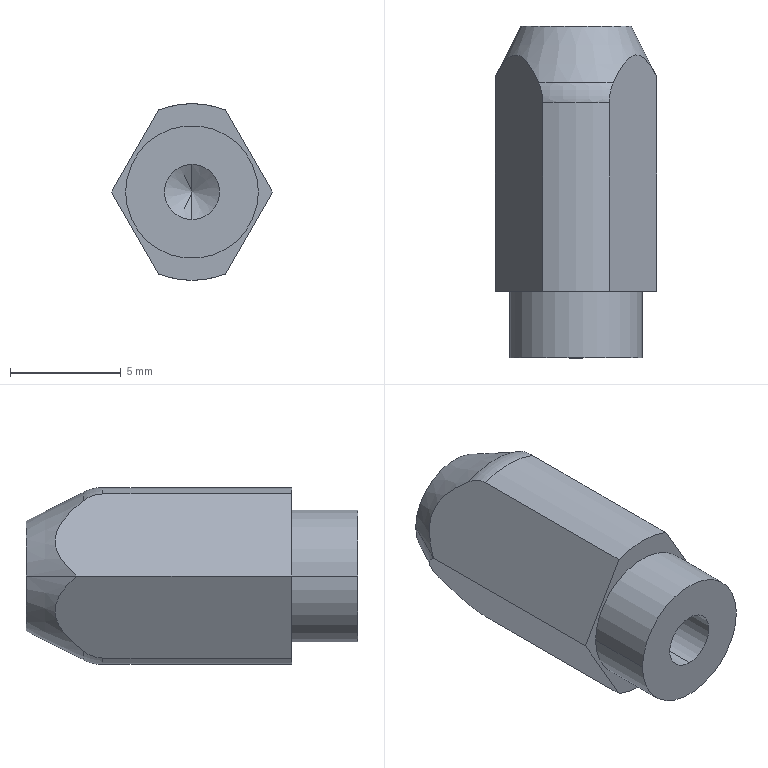Part | SolidWorks | features Fillet 1, HoleWzd 1, ICE 1, Revolution 1 | 1 solid | 19 faces | box 7.282 x 15 x 8 mm | volume 482.004 mm3 | plane 7 | cylinder 6 | cone 4 | torus 2 | commonest cylinder face diameters 2.5 x2 6 x2 8 x2
STEP:
#1=CARTESIAN_POINT('',(0.,10.,1.25));
#2=VERTEX_POINT('',#1);
#3=CARTESIAN_POINT('',(0.,10.,-1.25));
#4=VERTEX_POINT('',#3);
#5=CARTESIAN_POINT('',(0.,10.,0.));
#6=DIRECTION('',(0.,-1.,0.));
#7=DIRECTION('',(0.,0.,-1.));
#8=AXIS2_PLACEMENT_3D('',#5,#6,#7);
#9=CIRCLE('',#8,1.25);
#10=EDGE_CURVE('',#2,#4,#9,.T.);
#11=ORIENTED_EDGE('',*,*,#10,.F.);
#12=CARTESIAN_POINT('',(0.,0.,1.25));
#13=VERTEX_POINT('',#12);
#14=CARTESIAN_POINT('',(0.,0.,1.25));
#15=DIRECTION('',(0.,-1.,0.));
#16=VECTOR('',#15,1000.);
#17=LINE('',#14,#16);
#18=EDGE_CURVE('',#2,#13,#17,.T.);
#19=ORIENTED_EDGE('',*,*,#18,.T.);
#20=CARTESIAN_POINT('',(0.,0.,-1.25));
#21=VERTEX_POINT('',#20);
#22=CARTESIAN_POINT('',(0.,0.,0.));
#23=DIRECTION('',(0.,-1.,0.));
#24=DIRECTION('',(0.,0.,-1.));
#25=AXIS2_PLACEMENT_3D('',#22,#23,#24);
#26=CIRCLE('',#25,1.25);
#27=EDGE_CURVE('',#13,#21,#26,.T.);
#28=ORIENTED_EDGE('',*,*,#27,.T.);
#29=CARTESIAN_POINT('',(0.,0.,-1.25));
#30=DIRECTION('',(0.,-1.,0.));
#31=VECTOR('',#30,1000.);
#32=LINE('',#29,#31);
#33=EDGE_CURVE('',#4,#21,#32,.T.);
#34=ORIENTED_EDGE('',*,*,#33,.F.);
#35=EDGE_LOOP('',(#11,#19,#28,#34));
#36=FACE_OUTER_BOUND('',#35,.T.);
#37=CARTESIAN_POINT('',(0.,0.,0.));
#38=DIRECTION('',(0.,-1.,0.));
#39=DIRECTION('',(0.,0.,-1.));
#40=AXIS2_PLACEMENT_3D('',#37,#38,#39);
#41=CYLINDRICAL_SURFACE('',#40,1.25);
#42=ADVANCED_FACE('',(#36),#41,.F.);
#43=CARTESIAN_POINT('',(0.,10.751,0.));
#44=VERTEX_POINT('',#43);
#45=CARTESIAN_POINT('',(0.,10.,-1.25));
#46=DIRECTION('',(0.,-0.515,-0.8572));
#47=VECTOR('',#46,1000.);
#48=LINE('',#45,#47);
#49=EDGE_CURVE('',#44,#4,#48,.T.);
#50=ORIENTED_EDGE('',*,*,#49,.F.);
#51=CARTESIAN_POINT('',(0.,10.,1.25));
#52=DIRECTION('',(0.,-0.515,0.8572));
#53=VECTOR('',#52,1000.);
#54=LINE('',#51,#53);
#55=EDGE_CURVE('',#44,#2,#54,.T.);
#56=ORIENTED_EDGE('',*,*,#55,.T.);
#57=ORIENTED_EDGE('',*,*,#10,.T.);
#58=EDGE_LOOP('',(#50,#56,#57));
#59=FACE_OUTER_BOUND('',#58,.T.);
#60=CARTESIAN_POINT('',(0.,10.,0.));
#61=DIRECTION('',(0.,-1.,0.));
#62=DIRECTION('',(0.,0.,-1.));
#63=AXIS2_PLACEMENT_3D('',#60,#61,#62);
#64=CONICAL_SURFACE('',#63,1.25,1.03);
#65=ADVANCED_FACE('',(#59),#64,.F.);
#66=CARTESIAN_POINT('',(3.,3.,0.));
#67=VERTEX_POINT('',#66);
#68=CARTESIAN_POINT('',(-3.,3.,0.));
#69=VERTEX_POINT('',#68);
#70=CARTESIAN_POINT('',(0.,3.,0.));
#71=DIRECTION('',(0.,-1.,0.));
#72=DIRECTION('',(1.,0.,0.));
#73=AXIS2_PLACEMENT_3D('',#70,#71,#72);
#74=CIRCLE('',#73,3.);
#75=EDGE_CURVE('',#67,#69,#74,.T.);
#76=ORIENTED_EDGE('',*,*,#75,.T.);
#77=CARTESIAN_POINT('',(-3.,0.,0.));
#78=VERTEX_POINT('',#77);
#79=CARTESIAN_POINT('',(-3.,0.,0.));
#80=DIRECTION('',(0.,-1.,0.));
#81=VECTOR('',#80,1000.);
#82=LINE('',#79,#81);
#83=EDGE_CURVE('',#69,#78,#82,.T.);
#84=ORIENTED_EDGE('',*,*,#83,.T.);
#85=CARTESIAN_POINT('',(3.,0.,0.));
#86=VERTEX_POINT('',#85);
#87=CARTESIAN_POINT('',(0.,0.,0.));
#88=DIRECTION('',(0.,-1.,0.));
#89=DIRECTION('',(1.,0.,0.));
#90=AXIS2_PLACEMENT_3D('',#87,#88,#89);
#91=CIRCLE('',#90,3.);
#92=EDGE_CURVE('',#86,#78,#91,.T.);
#93=ORIENTED_EDGE('',*,*,#92,.F.);
#94=CARTESIAN_POINT('',(3.,0.,0.));
#95=DIRECTION('',(0.,-1.,0.));
#96=VECTOR('',#95,1000.);
#97=LINE('',#94,#96);
#98=EDGE_CURVE('',#67,#86,#97,.T.);
#99=ORIENTED_EDGE('',*,*,#98,.F.);
#100=EDGE_LOOP('',(#76,#84,#93,#99));
#101=FACE_OUTER_BOUND('',#100,.T.);
#102=CARTESIAN_POINT('',(0.,0.,0.));
#103=DIRECTION('',(0.,-1.,0.));
#104=DIRECTION('',(1.,0.,0.));
#105=AXIS2_PLACEMENT_3D('',#102,#103,#104);
#106=CYLINDRICAL_SURFACE('',#105,3.);
#107=ADVANCED_FACE('',(#101),#106,.T.);
#108=CARTESIAN_POINT('',(2.5,15.,0.));
#109=VERTEX_POINT('',#108);
#110=CARTESIAN_POINT('',(-2.5,15.,0.));
#111=VERTEX_POINT('',#110);
#112=CARTESIAN_POINT('',(0.,15.,0.));
#113=DIRECTION('',(0.,-1.,0.));
#114=DIRECTION('',(1.,0.,0.));
#115=AXIS2_PLACEMENT_3D('',#112,#113,#114);
#116=CIRCLE('',#115,2.5);
#117=EDGE_CURVE('',#109,#111,#116,.T.);
#118=ORIENTED_EDGE('',*,*,#117,.T.);
#119=CARTESIAN_POINT('',(-3.641,12.718,0.));
#120=VERTEX_POINT('',#119);
#121=CARTESIAN_POINT('',(-4.,12.,0.));
#122=DIRECTION('',(-0.4472,-0.8944,0.));
#123=VECTOR('',#122,1000.);
#124=LINE('',#121,#123);
#125=EDGE_CURVE('',#111,#120,#124,.T.);
#126=ORIENTED_EDGE('',*,*,#125,.T.);
#127=CARTESIAN_POINT('',(-1.68,12.422,3.396));
#128=VERTEX_POINT('',#127);
#129=CARTESIAN_POINT('',(-1.68,12.422,3.396));
#130=CARTESIAN_POINT('',(-1.745,12.566,3.284));
#131=CARTESIAN_POINT('',(-1.812,12.705,3.168));
#132=CARTESIAN_POINT('',(-1.953,12.972,2.924));
#133=CARTESIAN_POINT('',(-2.026,13.099,2.796));
#134=CARTESIAN_POINT('',(-2.182,13.329,2.527));
#135=CARTESIAN_POINT('',(-2.264,13.432,2.385));
#136=CARTESIAN_POINT('',(-2.44,13.597,2.079));
#137=CARTESIAN_POINT('',(-2.533,13.656,1.92));
#138=CARTESIAN_POINT('',(-2.727,13.706,1.584));
#139=CARTESIAN_POINT('',(-2.823,13.694,1.417));
#140=CARTESIAN_POINT('',(-3.013,13.605,1.088));
#141=CARTESIAN_POINT('',(-3.102,13.53,0.9338));
#142=CARTESIAN_POINT('',(-3.271,13.342,0.6408));
#143=CARTESIAN_POINT('',(-3.351,13.229,0.5025));
#144=CARTESIAN_POINT('',(-3.501,12.986,0.2421));
#145=CARTESIAN_POINT('',(-3.572,12.855,0.1188));
#146=CARTESIAN_POINT('',(-3.641,12.718,0.));
#147=B_SPLINE_CURVE_WITH_KNOTS('',3,(#129,#130,#131,#132,#133,#134,#135,#136,#137,#138,#139,#140,#141,#142,#143,#144,#145,#146),.UNSPECIFIED.,.F.,.F.,(4,2,2,2,2,2,2,2,4),(0.0005548,0.001135,0.001715,0.002295,0.002875,0.003455,0.004035,0.004615,0.005195),.UNSPECIFIED.);
#148=EDGE_CURVE('',#128,#120,#147,.T.);
#149=ORIENTED_EDGE('',*,*,#148,.F.);
#150=CARTESIAN_POINT('',(1.68,12.422,3.396));
#151=VERTEX_POINT('',#150);
#152=CARTESIAN_POINT('',(0.,12.422,0.));
#153=DIRECTION('',(0.,1.,0.));
#154=DIRECTION('',(-1.,0.,0.));
#155=AXIS2_PLACEMENT_3D('',#152,#153,#154);
#156=CIRCLE('',#155,3.789);
#157=EDGE_CURVE('',#128,#151,#156,.T.);
#158=ORIENTED_EDGE('',*,*,#157,.T.);
#159=CARTESIAN_POINT('',(3.641,12.718,0.));
#160=VERTEX_POINT('',#159);
#161=CARTESIAN_POINT('',(3.641,12.718,0.));
#162=CARTESIAN_POINT('',(3.572,12.856,0.1189));
#163=CARTESIAN_POINT('',(3.501,12.986,0.242));
#164=CARTESIAN_POINT('',(3.351,13.228,0.5015));
#165=CARTESIAN_POINT('',(3.273,13.339,0.6376));
#166=CARTESIAN_POINT('',(3.103,13.529,0.9318));
#167=CARTESIAN_POINT('',(3.012,13.605,1.089));
#168=CARTESIAN_POINT('',(2.87,13.672,1.335));
#169=CARTESIAN_POINT('',(2.821,13.686,1.42));
#170=CARTESIAN_POINT('',(2.724,13.697,1.587));
#171=CARTESIAN_POINT('',(2.676,13.693,1.671));
#172=CARTESIAN_POINT('',(2.58,13.668,1.837));
#173=CARTESIAN_POINT('',(2.532,13.647,1.921));
#174=CARTESIAN_POINT('',(2.439,13.589,2.082));
#175=CARTESIAN_POINT('',(2.394,13.554,2.16));
#176=CARTESIAN_POINT('',(2.262,13.43,2.388));
#177=CARTESIAN_POINT('',(2.179,13.325,2.532));
#178=CARTESIAN_POINT('',(1.947,12.981,2.935));
#179=CARTESIAN_POINT('',(1.81,12.71,3.172));
#180=CARTESIAN_POINT('',(1.68,12.422,3.396));
#181=B_SPLINE_CURVE_WITH_KNOTS('',3,(#161,#162,#163,#164,#165,#166,#167,#168,#169,#170,#171,#172,#173,#174,#175,#176,#177,#178,#179,#180),.UNSPECIFIED.,.F.,.F.,(4,2,2,2,2,2,2,2,2,4),(0.000000324,0.0005776,0.001155,0.001732,0.002021,0.002309,0.002598,0.002887,0.003464,0.004619),.UNSPECIFIED.);
#182=EDGE_CURVE('',#160,#151,#181,.T.);
#183=ORIENTED_EDGE('',*,*,#182,.F.);
#184=CARTESIAN_POINT('',(4.,12.,0.));
#185=DIRECTION('',(0.4472,-0.8944,0.));
#186=VECTOR('',#185,1000.);
#187=LINE('',#184,#186);
#188=EDGE_CURVE('',#109,#160,#187,.T.);
#189=ORIENTED_EDGE('',*,*,#188,.F.);
#190=EDGE_LOOP('',(#118,#126,#149,#158,#183,#189));
#191=FACE_OUTER_BOUND('',#190,.T.);
#192=CARTESIAN_POINT('',(0.,12.,0.));
#193=DIRECTION('',(0.,-1.,0.));
#194=DIRECTION('',(1.,0.,0.));
#195=AXIS2_PLACEMENT_3D('',#192,#193,#194);
#196=CONICAL_SURFACE('',#195,4.,0.4636);
#197=ADVANCED_FACE('',(#191),#196,.T.);
#198=CARTESIAN_POINT('',(1.5,3.,3.708));
#199=VERTEX_POINT('',#198);
#200=CARTESIAN_POINT('',(1.5,11.528,3.708));
#201=VERTEX_POINT('',#200);
#202=CARTESIAN_POINT('',(1.5,0.,3.708));
#203=DIRECTION('',(0.,1.,0.));
#204=VECTOR('',#203,1000.);
#205=LINE('',#202,#204);
#206=EDGE_CURVE('',#199,#201,#205,.T.);
#207=ORIENTED_EDGE('',*,*,#206,.T.);
#208=CARTESIAN_POINT('',(-1.5,11.528,3.708));
#209=VERTEX_POINT('',#208);
#210=CARTESIAN_POINT('',(0.,11.528,0.));
#211=DIRECTION('',(0.,-1.,0.));
#212=DIRECTION('',(-1.,0.,0.));
#213=AXIS2_PLACEMENT_3D('',#210,#211,#212);
#214=CIRCLE('',#213,4.);
#215=EDGE_CURVE('',#201,#209,#214,.T.);
#216=ORIENTED_EDGE('',*,*,#215,.T.);
#217=CARTESIAN_POINT('',(-1.5,3.,3.708));
#218=VERTEX_POINT('',#217);
#219=CARTESIAN_POINT('',(-1.5,0.,3.708));
#220=DIRECTION('',(0.,1.,0.));
#221=VECTOR('',#220,1000.);
#222=LINE('',#219,#221);
#223=EDGE_CURVE('',#218,#209,#222,.T.);
#224=ORIENTED_EDGE('',*,*,#223,.F.);
#225=CARTESIAN_POINT('',(0.,3.,0.));
#226=DIRECTION('',(0.,-1.,0.));
#227=DIRECTION('',(1.,0.,0.));
#228=AXIS2_PLACEMENT_3D('',#225,#226,#227);
#229=CIRCLE('',#228,4.);
#230=EDGE_CURVE('',#199,#218,#229,.T.);
#231=ORIENTED_EDGE('',*,*,#230,.F.);
#232=EDGE_LOOP('',(#207,#216,#224,#231));
#233=FACE_OUTER_BOUND('',#232,.T.);
#234=CARTESIAN_POINT('',(0.,0.,0.));
#235=DIRECTION('',(0.,-1.,0.));
#236=DIRECTION('',(1.,0.,0.));
#237=AXIS2_PLACEMENT_3D('',#234,#235,#236);
#238=CYLINDRICAL_SURFACE('',#237,4.);
#239=ADVANCED_FACE('',(#233),#238,.T.);
#240=CARTESIAN_POINT('',(0.,0.,0.));
#241=DIRECTION('',(0.,-1.,0.));
#242=DIRECTION('',(0.,0.,-1.));
#243=AXIS2_PLACEMENT_3D('',#240,#241,#242);
#244=CIRCLE('',#243,1.25);
#245=EDGE_CURVE('',#21,#13,#244,.T.);
#246=ORIENTED_EDGE('',*,*,#245,.F.);
#247=ORIENTED_EDGE('',*,*,#27,.F.);
#248=EDGE_LOOP('',(#246,#247));
#249=FACE_BOUND('',#248,.T.);
#250=ORIENTED_EDGE('',*,*,#92,.T.);
#251=CARTESIAN_POINT('',(0.,0.,0.));
#252=DIRECTION('',(0.,-1.,0.));
#253=DIRECTION('',(1.,0.,0.));
#254=AXIS2_PLACEMENT_3D('',#251,#252,#253);
#255=CIRCLE('',#254,3.);
#256=EDGE_CURVE('',#78,#86,#255,.T.);
#257=ORIENTED_EDGE('',*,*,#256,.T.);
#258=EDGE_LOOP('',(#250,#257));
#259=FACE_OUTER_BOUND('',#258,.T.);
#260=CARTESIAN_POINT('',(3.,0.,0.));
#261=DIRECTION('',(0.,-1.,0.));
#262=DIRECTION('',(1.,0.,0.));
#263=AXIS2_PLACEMENT_3D('',#260,#261,#262);
#264=PLANE('',#263);
#265=ADVANCED_FACE('',(#249,#259),#264,.T.);
#266=ORIENTED_EDGE('',*,*,#117,.F.);
#267=CARTESIAN_POINT('',(0.,15.,0.));
#268=DIRECTION('',(0.,-1.,0.));
#269=DIRECTION('',(1.,0.,0.));
#270=AXIS2_PLACEMENT_3D('',#267,#268,#269);
#271=CIRCLE('',#270,2.5);
#272=EDGE_CURVE('',#111,#109,#271,.T.);
#273=ORIENTED_EDGE('',*,*,#272,.F.);
#274=EDGE_LOOP('',(#266,#273));
#275=FACE_OUTER_BOUND('',#274,.T.);
#276=CARTESIAN_POINT('',(0.,15.,0.));
#277=DIRECTION('',(0.,1.,0.));
#278=DIRECTION('',(-1.,0.,0.));
#279=AXIS2_PLACEMENT_3D('',#276,#277,#278);
#280=PLANE('',#279);
#281=ADVANCED_FACE('',(#275),#280,.T.);
#282=ORIENTED_EDGE('',*,*,#125,.F.);
#283=ORIENTED_EDGE('',*,*,#272,.T.);
#284=ORIENTED_EDGE('',*,*,#188,.T.);
#285=CARTESIAN_POINT('',(1.68,12.422,-3.396));
#286=VERTEX_POINT('',#285);
#287=CARTESIAN_POINT('',(1.68,12.422,-3.396));
#288=CARTESIAN_POINT('',(1.745,12.566,-3.284));
#289=CARTESIAN_POINT('',(1.812,12.705,-3.168));
#290=CARTESIAN_POINT('',(1.953,12.972,-2.924));
#291=CARTESIAN_POINT('',(2.026,13.099,-2.796));
#292=CARTESIAN_POINT('',(2.182,13.329,-2.527));
#293=CARTESIAN_POINT('',(2.264,13.432,-2.385));
#294=CARTESIAN_POINT('',(2.44,13.597,-2.079));
#295=CARTESIAN_POINT('',(2.533,13.656,-1.92));
#296=CARTESIAN_POINT('',(2.727,13.706,-1.584));
#297=CARTESIAN_POINT('',(2.823,13.694,-1.417));
#298=CARTESIAN_POINT('',(3.013,13.605,-1.088));
#299=CARTESIAN_POINT('',(3.102,13.53,-0.9338));
#300=CARTESIAN_POINT('',(3.271,13.342,-0.6408));
#301=CARTESIAN_POINT('',(3.351,13.229,-0.5025));
#302=CARTESIAN_POINT('',(3.501,12.986,-0.2421));
#303=CARTESIAN_POINT('',(3.572,12.855,-0.1188));
#304=CARTESIAN_POINT('',(3.641,12.718,0.));
#305=B_SPLINE_CURVE_WITH_KNOTS('',3,(#287,#288,#289,#290,#291,#292,#293,#294,#295,#296,#297,#298,#299,#300,#301,#302,#303,#304),.UNSPECIFIED.,.F.,.F.,(4,2,2,2,2,2,2,2,4),(0.0005548,0.001135,0.001715,0.002295,0.002875,0.003455,0.004035,0.004615,0.005195),.UNSPECIFIED.);
#306=EDGE_CURVE('',#286,#160,#305,.T.);
#307=ORIENTED_EDGE('',*,*,#306,.F.);
#308=CARTESIAN_POINT('',(-1.68,12.422,-3.396));
#309=VERTEX_POINT('',#308);
#310=CARTESIAN_POINT('',(0.,12.422,0.));
#311=DIRECTION('',(0.,1.,0.));
#312=DIRECTION('',(-1.,0.,0.));
#313=AXIS2_PLACEMENT_3D('',#310,#311,#312);
#314=CIRCLE('',#313,3.789);
#315=EDGE_CURVE('',#286,#309,#314,.T.);
#316=ORIENTED_EDGE('',*,*,#315,.T.);
#317=CARTESIAN_POINT('',(-3.641,12.718,0.));
#318=CARTESIAN_POINT('',(-3.572,12.856,-0.1189));
#319=CARTESIAN_POINT('',(-3.501,12.986,-0.242));
#320=CARTESIAN_POINT('',(-3.351,13.228,-0.5015));
#321=CARTESIAN_POINT('',(-3.273,13.339,-0.6376));
#322=CARTESIAN_POINT('',(-3.103,13.529,-0.9318));
#323=CARTESIAN_POINT('',(-3.012,13.605,-1.089));
#324=CARTESIAN_POINT('',(-2.87,13.672,-1.335));
#325=CARTESIAN_POINT('',(-2.821,13.686,-1.42));
#326=CARTESIAN_POINT('',(-2.724,13.697,-1.587));
#327=CARTESIAN_POINT('',(-2.676,13.693,-1.671));
#328=CARTESIAN_POINT('',(-2.58,13.668,-1.837));
#329=CARTESIAN_POINT('',(-2.532,13.647,-1.921));
#330=CARTESIAN_POINT('',(-2.439,13.589,-2.082));
#331=CARTESIAN_POINT('',(-2.394,13.554,-2.16));
#332=CARTESIAN_POINT('',(-2.262,13.43,-2.388));
#333=CARTESIAN_POINT('',(-2.179,13.325,-2.532));
#334=CARTESIAN_POINT('',(-1.947,12.981,-2.935));
#335=CARTESIAN_POINT('',(-1.81,12.71,-3.172));
#336=CARTESIAN_POINT('',(-1.68,12.422,-3.396));
#337=B_SPLINE_CURVE_WITH_KNOTS('',3,(#317,#318,#319,#320,#321,#322,#323,#324,#325,#326,#327,#328,#329,#330,#331,#332,#333,#334,#335,#336),.UNSPECIFIED.,.F.,.F.,(4,2,2,2,2,2,2,2,2,4),(0.000000324,0.0005776,0.001155,0.001732,0.002021,0.002309,0.002598,0.002887,0.003464,0.004619),.UNSPECIFIED.);
#338=EDGE_CURVE('',#120,#309,#337,.T.);
#339=ORIENTED_EDGE('',*,*,#338,.F.);
#340=EDGE_LOOP('',(#282,#283,#284,#307,#316,#339));
#341=FACE_OUTER_BOUND('',#340,.T.);
#342=CARTESIAN_POINT('',(0.,12.,0.));
#343=DIRECTION('',(0.,-1.,0.));
#344=DIRECTION('',(1.,0.,0.));
#345=AXIS2_PLACEMENT_3D('',#342,#343,#344);
#346=CONICAL_SURFACE('',#345,4.,0.4636);
#347=ADVANCED_FACE('',(#341),#346,.T.);
#348=CARTESIAN_POINT('',(-1.5,3.,-3.708));
#349=VERTEX_POINT('',#348);
#350=CARTESIAN_POINT('',(-1.5,11.528,-3.708));
#351=VERTEX_POINT('',#350);
#352=CARTESIAN_POINT('',(-1.5,0.,-3.708));
#353=DIRECTION('',(0.,1.,0.));
#354=VECTOR('',#353,1000.);
#355=LINE('',#352,#354);
#356=EDGE_CURVE('',#349,#351,#355,.T.);
#357=ORIENTED_EDGE('',*,*,#356,.T.);
#358=CARTESIAN_POINT('',(1.5,11.528,-3.708));
#359=VERTEX_POINT('',#358);
#360=CARTESIAN_POINT('',(0.,11.528,0.));
#361=DIRECTION('',(0.,-1.,0.));
#362=DIRECTION('',(-1.,0.,0.));
#363=AXIS2_PLACEMENT_3D('',#360,#361,#362);
#364=CIRCLE('',#363,4.);
#365=EDGE_CURVE('',#351,#359,#364,.T.);
#366=ORIENTED_EDGE('',*,*,#365,.T.);
#367=CARTESIAN_POINT('',(1.5,3.,-3.708));
#368=VERTEX_POINT('',#367);
#369=CARTESIAN_POINT('',(1.5,0.,-3.708));
#370=DIRECTION('',(0.,1.,0.));
#371=VECTOR('',#370,1000.);
#372=LINE('',#369,#371);
#373=EDGE_CURVE('',#368,#359,#372,.T.);
#374=ORIENTED_EDGE('',*,*,#373,.F.);
#375=CARTESIAN_POINT('',(0.,3.,0.));
#376=DIRECTION('',(0.,-1.,0.));
#377=DIRECTION('',(1.,0.,0.));
#378=AXIS2_PLACEMENT_3D('',#375,#376,#377);
#379=CIRCLE('',#378,4.);
#380=EDGE_CURVE('',#349,#368,#379,.T.);
#381=ORIENTED_EDGE('',*,*,#380,.F.);
#382=EDGE_LOOP('',(#357,#366,#374,#381));
#383=FACE_OUTER_BOUND('',#382,.T.);
#384=CARTESIAN_POINT('',(0.,0.,0.));
#385=DIRECTION('',(0.,-1.,0.));
#386=DIRECTION('',(1.,0.,0.));
#387=AXIS2_PLACEMENT_3D('',#384,#385,#386);
#388=CYLINDRICAL_SURFACE('',#387,4.);
#389=ADVANCED_FACE('',(#383),#388,.T.);
#390=CARTESIAN_POINT('',(-3.641,3.,0.));
#391=VERTEX_POINT('',#390);
#392=CARTESIAN_POINT('',(-1.731,3.,3.309));
#393=DIRECTION('',(0.5,0.,0.866));
#394=VECTOR('',#393,1000.);
#395=LINE('',#392,#394);
#396=EDGE_CURVE('',#391,#218,#395,.T.);
#397=ORIENTED_EDGE('',*,*,#396,.F.);
#398=CARTESIAN_POINT('',(-1.731,3.,-3.309));
#399=DIRECTION('',(-0.5,0.,0.866));
#400=VECTOR('',#399,1000.);
#401=LINE('',#398,#400);
#402=EDGE_CURVE('',#349,#391,#401,.T.);
#403=ORIENTED_EDGE('',*,*,#402,.F.);
#404=ORIENTED_EDGE('',*,*,#380,.T.);
#405=CARTESIAN_POINT('',(3.641,3.,0.));
#406=VERTEX_POINT('',#405);
#407=CARTESIAN_POINT('',(3.731,3.,0.1555));
#408=DIRECTION('',(-0.5,0.,-0.866));
#409=VECTOR('',#408,1000.);
#410=LINE('',#407,#409);
#411=EDGE_CURVE('',#406,#368,#410,.T.);
#412=ORIENTED_EDGE('',*,*,#411,.F.);
#413=CARTESIAN_POINT('',(3.731,3.,-0.1555));
#414=DIRECTION('',(0.5,0.,-0.866));
#415=VECTOR('',#414,1000.);
#416=LINE('',#413,#415);
#417=EDGE_CURVE('',#199,#406,#416,.T.);
#418=ORIENTED_EDGE('',*,*,#417,.F.);
#419=ORIENTED_EDGE('',*,*,#230,.T.);
#420=EDGE_LOOP('',(#397,#403,#404,#412,#418,#419));
#421=FACE_OUTER_BOUND('',#420,.T.);
#422=ORIENTED_EDGE('',*,*,#75,.F.);
#423=CARTESIAN_POINT('',(0.,3.,0.));
#424=DIRECTION('',(0.,-1.,0.));
#425=DIRECTION('',(1.,0.,0.));
#426=AXIS2_PLACEMENT_3D('',#423,#424,#425);
#427=CIRCLE('',#426,3.);
#428=EDGE_CURVE('',#69,#67,#427,.T.);
#429=ORIENTED_EDGE('',*,*,#428,.F.);
#430=EDGE_LOOP('',(#422,#429));
#431=FACE_BOUND('',#430,.T.);
#432=CARTESIAN_POINT('',(4.,3.,0.));
#433=DIRECTION('',(0.,-1.,0.));
#434=DIRECTION('',(1.,0.,0.));
#435=AXIS2_PLACEMENT_3D('',#432,#433,#434);
#436=PLANE('',#435);
#437=ADVANCED_FACE('',(#421,#431),#436,.T.);
#438=ORIENTED_EDGE('',*,*,#83,.F.);
#439=ORIENTED_EDGE('',*,*,#428,.T.);
#440=ORIENTED_EDGE('',*,*,#98,.T.);
#441=ORIENTED_EDGE('',*,*,#256,.F.);
#442=EDGE_LOOP('',(#438,#439,#440,#441));
#443=FACE_OUTER_BOUND('',#442,.T.);
#444=CARTESIAN_POINT('',(0.,0.,0.));
#445=DIRECTION('',(0.,-1.,0.));
#446=DIRECTION('',(1.,0.,0.));
#447=AXIS2_PLACEMENT_3D('',#444,#445,#446);
#448=CYLINDRICAL_SURFACE('',#447,3.);
#449=ADVANCED_FACE('',(#443),#448,.T.);
#450=ORIENTED_EDGE('',*,*,#55,.F.);
#451=ORIENTED_EDGE('',*,*,#49,.T.);
#452=CARTESIAN_POINT('',(0.,10.,0.));
#453=DIRECTION('',(0.,-1.,0.));
#454=DIRECTION('',(0.,0.,-1.));
#455=AXIS2_PLACEMENT_3D('',#452,#453,#454);
#456=CIRCLE('',#455,1.25);
#457=EDGE_CURVE('',#4,#2,#456,.T.);
#458=ORIENTED_EDGE('',*,*,#457,.T.);
#459=EDGE_LOOP('',(#450,#451,#458));
#460=FACE_OUTER_BOUND('',#459,.T.);
#461=CARTESIAN_POINT('',(0.,10.,0.));
#462=DIRECTION('',(0.,-1.,0.));
#463=DIRECTION('',(0.,0.,-1.));
#464=AXIS2_PLACEMENT_3D('',#461,#462,#463);
#465=CONICAL_SURFACE('',#464,1.25,1.03);
#466=ADVANCED_FACE('',(#460),#465,.F.);
#467=ORIENTED_EDGE('',*,*,#18,.F.);
#468=ORIENTED_EDGE('',*,*,#457,.F.);
#469=ORIENTED_EDGE('',*,*,#33,.T.);
#470=ORIENTED_EDGE('',*,*,#245,.T.);
#471=EDGE_LOOP('',(#467,#468,#469,#470));
#472=FACE_OUTER_BOUND('',#471,.T.);
#473=CARTESIAN_POINT('',(0.,0.,0.));
#474=DIRECTION('',(0.,-1.,0.));
#475=DIRECTION('',(0.,0.,-1.));
#476=AXIS2_PLACEMENT_3D('',#473,#474,#475);
#477=CYLINDRICAL_SURFACE('',#476,1.25);
#478=ADVANCED_FACE('',(#472),#477,.F.);
#479=ORIENTED_EDGE('',*,*,#182,.T.);
#480=CARTESIAN_POINT('',(1.68,12.422,3.396));
#481=CARTESIAN_POINT('',(1.625,12.299,3.492));
#482=CARTESIAN_POINT('',(1.58,12.161,3.57));
#483=CARTESIAN_POINT('',(1.517,11.856,3.679));
#484=CARTESIAN_POINT('',(1.5,11.694,3.708));
#485=CARTESIAN_POINT('',(1.5,11.528,3.708));
#486=B_SPLINE_CURVE_WITH_KNOTS('',3,(#480,#481,#482,#483,#484,#485),.UNSPECIFIED.,.F.,.F.,(4,2,4),(0.,0.0004913,0.0009825),.UNSPECIFIED.);
#487=EDGE_CURVE('',#151,#201,#486,.T.);
#488=ORIENTED_EDGE('',*,*,#487,.T.);
#489=ORIENTED_EDGE('',*,*,#206,.F.);
#490=ORIENTED_EDGE('',*,*,#417,.T.);
#491=CARTESIAN_POINT('',(3.641,0.,0.));
#492=DIRECTION('',(0.,1.,0.));
#493=VECTOR('',#492,1000.);
#494=LINE('',#491,#493);
#495=EDGE_CURVE('',#406,#160,#494,.T.);
#496=ORIENTED_EDGE('',*,*,#495,.T.);
#497=EDGE_LOOP('',(#479,#488,#489,#490,#496));
#498=FACE_OUTER_BOUND('',#497,.T.);
#499=CARTESIAN_POINT('',(3.641,0.,0.));
#500=DIRECTION('',(-0.866,0.,-0.5));
#501=DIRECTION('',(-0.5,0.,0.866));
#502=AXIS2_PLACEMENT_3D('',#499,#500,#501);
#503=PLANE('',#502);
#504=ADVANCED_FACE('',(#498),#503,.F.);
#505=ORIENTED_EDGE('',*,*,#373,.T.);
#506=CARTESIAN_POINT('',(1.5,11.528,-3.708));
#507=CARTESIAN_POINT('',(1.5,11.694,-3.708));
#508=CARTESIAN_POINT('',(1.517,11.855,-3.679));
#509=CARTESIAN_POINT('',(1.58,12.161,-3.57));
#510=CARTESIAN_POINT('',(1.625,12.299,-3.492));
#511=CARTESIAN_POINT('',(1.68,12.422,-3.396));
#512=B_SPLINE_CURVE_WITH_KNOTS('',3,(#506,#507,#508,#509,#510,#511),.UNSPECIFIED.,.F.,.F.,(4,2,4),(0.,0.00049,0.00098),.UNSPECIFIED.);
#513=EDGE_CURVE('',#359,#286,#512,.T.);
#514=ORIENTED_EDGE('',*,*,#513,.T.);
#515=ORIENTED_EDGE('',*,*,#306,.T.);
#516=ORIENTED_EDGE('',*,*,#495,.F.);
#517=ORIENTED_EDGE('',*,*,#411,.T.);
#518=EDGE_LOOP('',(#505,#514,#515,#516,#517));
#519=FACE_OUTER_BOUND('',#518,.T.);
#520=CARTESIAN_POINT('',(1.5,0.,-3.708));
#521=DIRECTION('',(-0.866,0.,0.5));
#522=DIRECTION('',(0.5,0.,0.866));
#523=AXIS2_PLACEMENT_3D('',#520,#521,#522);
#524=PLANE('',#523);
#525=ADVANCED_FACE('',(#519),#524,.F.);
#526=ORIENTED_EDGE('',*,*,#223,.T.);
#527=CARTESIAN_POINT('',(-1.5,11.528,3.708));
#528=CARTESIAN_POINT('',(-1.5,11.694,3.708));
#529=CARTESIAN_POINT('',(-1.517,11.855,3.679));
#530=CARTESIAN_POINT('',(-1.58,12.161,3.57));
#531=CARTESIAN_POINT('',(-1.625,12.299,3.492));
#532=CARTESIAN_POINT('',(-1.68,12.422,3.396));
#533=B_SPLINE_CURVE_WITH_KNOTS('',3,(#527,#528,#529,#530,#531,#532),.UNSPECIFIED.,.F.,.F.,(4,2,4),(0.,0.00049,0.00098),.UNSPECIFIED.);
#534=EDGE_CURVE('',#209,#128,#533,.T.);
#535=ORIENTED_EDGE('',*,*,#534,.T.);
#536=ORIENTED_EDGE('',*,*,#148,.T.);
#537=CARTESIAN_POINT('',(-3.641,0.,0.));
#538=DIRECTION('',(0.,1.,0.));
#539=VECTOR('',#538,1000.);
#540=LINE('',#537,#539);
#541=EDGE_CURVE('',#391,#120,#540,.T.);
#542=ORIENTED_EDGE('',*,*,#541,.F.);
#543=ORIENTED_EDGE('',*,*,#396,.T.);
#544=EDGE_LOOP('',(#526,#535,#536,#542,#543));
#545=FACE_OUTER_BOUND('',#544,.T.);
#546=CARTESIAN_POINT('',(-3.641,0.,0.));
#547=DIRECTION('',(0.866,0.,-0.5));
#548=DIRECTION('',(-0.5,0.,-0.866));
#549=AXIS2_PLACEMENT_3D('',#546,#547,#548);
#550=PLANE('',#549);
#551=ADVANCED_FACE('',(#545),#550,.F.);
#552=ORIENTED_EDGE('',*,*,#338,.T.);
#553=CARTESIAN_POINT('',(-1.68,12.422,-3.396));
#554=CARTESIAN_POINT('',(-1.625,12.299,-3.492));
#555=CARTESIAN_POINT('',(-1.58,12.161,-3.57));
#556=CARTESIAN_POINT('',(-1.517,11.856,-3.679));
#557=CARTESIAN_POINT('',(-1.5,11.694,-3.708));
#558=CARTESIAN_POINT('',(-1.5,11.528,-3.708));
#559=B_SPLINE_CURVE_WITH_KNOTS('',3,(#553,#554,#555,#556,#557,#558),.UNSPECIFIED.,.F.,.F.,(4,2,4),(0.,0.0004913,0.0009825),.UNSPECIFIED.);
#560=EDGE_CURVE('',#309,#351,#559,.T.);
#561=ORIENTED_EDGE('',*,*,#560,.T.);
#562=ORIENTED_EDGE('',*,*,#356,.F.);
#563=ORIENTED_EDGE('',*,*,#402,.T.);
#564=ORIENTED_EDGE('',*,*,#541,.T.);
#565=EDGE_LOOP('',(#552,#561,#562,#563,#564));
#566=FACE_OUTER_BOUND('',#565,.T.);
#567=CARTESIAN_POINT('',(-1.5,0.,-3.708));
#568=DIRECTION('',(0.866,0.,0.5));
#569=DIRECTION('',(0.5,0.,-0.866));
#570=AXIS2_PLACEMENT_3D('',#567,#568,#569);
#571=PLANE('',#570);
#572=ADVANCED_FACE('',(#566),#571,.F.);
#573=ORIENTED_EDGE('',*,*,#560,.F.);
#574=ORIENTED_EDGE('',*,*,#315,.F.);
#575=ORIENTED_EDGE('',*,*,#513,.F.);
#576=ORIENTED_EDGE('',*,*,#365,.F.);
#577=EDGE_LOOP('',(#573,#574,#575,#576));
#578=FACE_OUTER_BOUND('',#577,.T.);
#579=CARTESIAN_POINT('',(0.,11.528,0.));
#580=DIRECTION('',(0.,1.,0.));
#581=DIRECTION('',(-1.,0.,0.));
#582=AXIS2_PLACEMENT_3D('',#579,#580,#581);
#583=TOROIDAL_SURFACE('',#582,2.,2.);
#584=ADVANCED_FACE('',(#578),#583,.T.);
#585=ORIENTED_EDGE('',*,*,#487,.F.);
#586=ORIENTED_EDGE('',*,*,#157,.F.);
#587=ORIENTED_EDGE('',*,*,#534,.F.);
#588=ORIENTED_EDGE('',*,*,#215,.F.);
#589=EDGE_LOOP('',(#585,#586,#587,#588));
#590=FACE_OUTER_BOUND('',#589,.T.);
#591=CARTESIAN_POINT('',(0.,11.528,0.));
#592=DIRECTION('',(0.,1.,0.));
#593=DIRECTION('',(-1.,0.,0.));
#594=AXIS2_PLACEMENT_3D('',#591,#592,#593);
#595=TOROIDAL_SURFACE('',#594,2.,2.);
#596=ADVANCED_FACE('',(#590),#595,.T.);
#597=CLOSED_SHELL('',(#42,#65,#107,#197,#239,#265,#281,#347,#389,#437,#449,#466,#478,#504,#525,#551,#572,#584,#596));
#598=MANIFOLD_SOLID_BREP('',#597);
#599=CARTESIAN_POINT('',(0.,0.,0.));
#600=DIRECTION('',(0.,0.,1.));
#601=DIRECTION('',(1.,0.,0.));
#602=AXIS2_PLACEMENT_3D('',#599,#600,#601);
#603=(LENGTH_UNIT()NAMED_UNIT(*)SI_UNIT(.MILLI.,.METRE.));
#604=UNCERTAINTY_MEASURE_WITH_UNIT(LENGTH_MEASURE(0.00001),#603,'','');
#605=(NAMED_UNIT(*)PLANE_ANGLE_UNIT()SI_UNIT($,.RADIAN.));
#606=(NAMED_UNIT(*)SI_UNIT($,.STERADIAN.)SOLID_ANGLE_UNIT());
#607=(GEOMETRIC_REPRESENTATION_CONTEXT(3)GLOBAL_UNCERTAINTY_ASSIGNED_CONTEXT((#604))GLOBAL_UNIT_ASSIGNED_CONTEXT((#603,#605,#606))REPRESENTATION_CONTEXT('',''));
#608=ADVANCED_BREP_SHAPE_REPRESENTATION('',(#598,#602),#607);